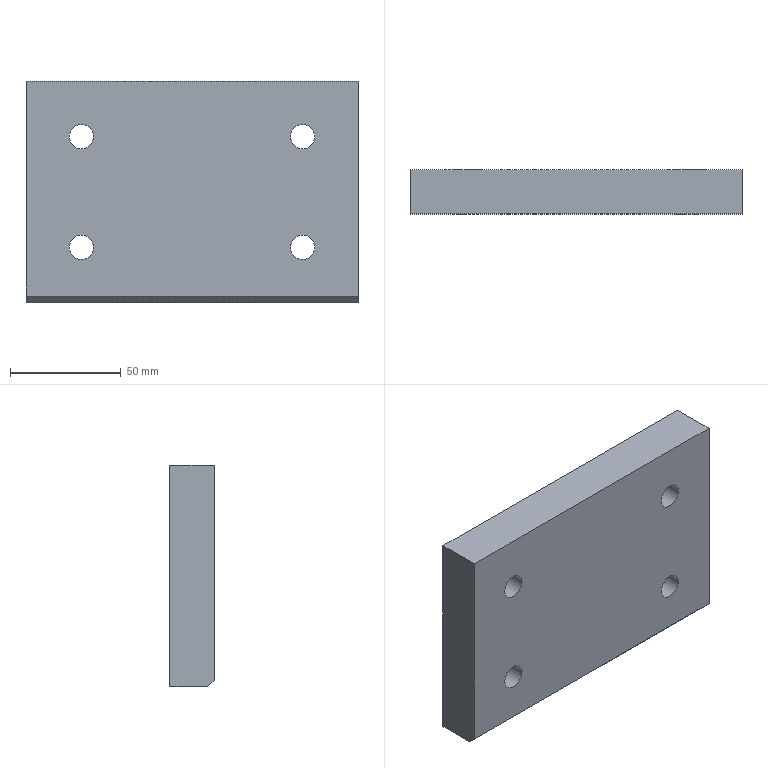Part | NX | features 103 2 | 1 solid | 19 faces | box 150 x 20 x 100 mm | volume 284739 mm3 | plane 11 | cylinder 8 | commonest cylinder face diameters 11 x4 17.5 x4
STEP:
#1=CARTESIAN_POINT('',(-1488.75,770.,-50.));
#2=VERTEX_POINT('',#1);
#3=CARTESIAN_POINT('',(-1480.,770.,-50.));
#4=DIRECTION('',(0.,1.,0.));
#5=DIRECTION('',(-1.,0.,0.));
#6=AXIS2_PLACEMENT_3D('',#3,#4,#5);
#7=CIRCLE('',#6,8.75);
#8=EDGE_CURVE('',#2,#2,#7,.T.);
#9=ORIENTED_EDGE('',*,*,#8,.F.);
#10=EDGE_LOOP('',(#9));
#11=FACE_BOUND('',#10,.T.);
#12=CARTESIAN_POINT('',(-1571.25,770.,0.000000001));
#13=VERTEX_POINT('',#12);
#14=CARTESIAN_POINT('',(-1580.,770.,0.000000001));
#15=DIRECTION('',(0.,-1.,0.));
#16=DIRECTION('',(1.,0.,0.));
#17=AXIS2_PLACEMENT_3D('',#14,#15,#16);
#18=CIRCLE('',#17,8.75);
#19=EDGE_CURVE('',#13,#13,#18,.F.);
#20=ORIENTED_EDGE('',*,*,#19,.F.);
#21=EDGE_LOOP('',(#20));
#22=FACE_BOUND('',#21,.T.);
#23=CARTESIAN_POINT('',(-1571.25,770.,-50.));
#24=VERTEX_POINT('',#23);
#25=CARTESIAN_POINT('',(-1580.,770.,-50.));
#26=DIRECTION('',(0.,-1.,0.));
#27=DIRECTION('',(1.,0.,0.));
#28=AXIS2_PLACEMENT_3D('',#25,#26,#27);
#29=CIRCLE('',#28,8.75);
#30=EDGE_CURVE('',#24,#24,#29,.F.);
#31=ORIENTED_EDGE('',*,*,#30,.F.);
#32=EDGE_LOOP('',(#31));
#33=FACE_BOUND('',#32,.T.);
#34=CARTESIAN_POINT('',(-1471.25,770.,0.000000001));
#35=VERTEX_POINT('',#34);
#36=CARTESIAN_POINT('',(-1480.,770.,0.000000001));
#37=DIRECTION('',(0.,-1.,0.));
#38=DIRECTION('',(1.,0.,0.));
#39=AXIS2_PLACEMENT_3D('',#36,#37,#38);
#40=CIRCLE('',#39,8.75);
#41=EDGE_CURVE('',#35,#35,#40,.F.);
#42=ORIENTED_EDGE('',*,*,#41,.F.);
#43=EDGE_LOOP('',(#42));
#44=FACE_BOUND('',#43,.T.);
#45=CARTESIAN_POINT('',(-1455.,770.,25.));
#46=VERTEX_POINT('',#45);
#47=CARTESIAN_POINT('',(-1455.,770.,-75.));
#48=VERTEX_POINT('',#47);
#49=CARTESIAN_POINT('',(-1455.,770.,-25.));
#50=DIRECTION('',(0.,0.,-1.));
#51=VECTOR('',#50,1000.);
#52=LINE('',#49,#51);
#53=EDGE_CURVE('',#46,#48,#52,.T.);
#54=ORIENTED_EDGE('',*,*,#53,.T.);
#55=CARTESIAN_POINT('',(-1605.,770.,-75.));
#56=VERTEX_POINT('',#55);
#57=CARTESIAN_POINT('',(-1530.,770.,-75.));
#58=DIRECTION('',(-1.,0.,0.));
#59=VECTOR('',#58,1000.);
#60=LINE('',#57,#59);
#61=EDGE_CURVE('',#48,#56,#60,.T.);
#62=ORIENTED_EDGE('',*,*,#61,.T.);
#63=CARTESIAN_POINT('',(-1605.,770.,25.));
#64=VERTEX_POINT('',#63);
#65=CARTESIAN_POINT('',(-1605.,770.,-25.));
#66=DIRECTION('',(0.,0.,1.));
#67=VECTOR('',#66,1000.);
#68=LINE('',#65,#67);
#69=EDGE_CURVE('',#56,#64,#68,.T.);
#70=ORIENTED_EDGE('',*,*,#69,.T.);
#71=CARTESIAN_POINT('',(-1530.,770.,25.));
#72=DIRECTION('',(1.,0.,0.));
#73=VECTOR('',#72,1000.);
#74=LINE('',#71,#73);
#75=EDGE_CURVE('',#64,#46,#74,.T.);
#76=ORIENTED_EDGE('',*,*,#75,.T.);
#77=EDGE_LOOP('',(#54,#62,#70,#76));
#78=FACE_BOUND('',#77,.T.);
#79=CARTESIAN_POINT('',(-1530.,770.,-25.));
#80=DIRECTION('',(0.,1.,0.));
#81=DIRECTION('',(1.,0.,0.));
#82=AXIS2_PLACEMENT_3D('',#79,#80,#81);
#83=PLANE('',#82);
#84=ADVANCED_FACE('',(#11,#22,#33,#44,#78),#83,.T.);
#85=CARTESIAN_POINT('',(-1605.,753.,-75.));
#86=VERTEX_POINT('',#85);
#87=CARTESIAN_POINT('',(-1605.,750.,-75.));
#88=DIRECTION('',(0.,1.,0.));
#89=VECTOR('',#88,1000.);
#90=LINE('',#87,#89);
#91=EDGE_CURVE('',#86,#56,#90,.T.);
#92=ORIENTED_EDGE('',*,*,#91,.T.);
#93=ORIENTED_EDGE('',*,*,#61,.F.);
#94=CARTESIAN_POINT('',(-1455.,753.,-75.));
#95=VERTEX_POINT('',#94);
#96=CARTESIAN_POINT('',(-1455.,750.,-75.));
#97=DIRECTION('',(0.,1.,0.));
#98=VECTOR('',#97,1000.);
#99=LINE('',#96,#98);
#100=EDGE_CURVE('',#95,#48,#99,.T.);
#101=ORIENTED_EDGE('',*,*,#100,.F.);
#102=CARTESIAN_POINT('',(-1530.,753.,-75.));
#103=DIRECTION('',(1.,0.,0.));
#104=VECTOR('',#103,1000.);
#105=LINE('',#102,#104);
#106=EDGE_CURVE('',#86,#95,#105,.T.);
#107=ORIENTED_EDGE('',*,*,#106,.F.);
#108=EDGE_LOOP('',(#92,#93,#101,#107));
#109=FACE_BOUND('',#108,.T.);
#110=CARTESIAN_POINT('',(-1530.,750.,-75.));
#111=DIRECTION('',(0.,0.,-1.));
#112=DIRECTION('',(0.,-1.,0.));
#113=AXIS2_PLACEMENT_3D('',#110,#111,#112);
#114=PLANE('',#113);
#115=ADVANCED_FACE('',(#109),#114,.T.);
#116=CARTESIAN_POINT('',(-1605.,750.,25.));
#117=VERTEX_POINT('',#116);
#118=CARTESIAN_POINT('',(-1605.,750.,-72.));
#119=VERTEX_POINT('',#118);
#120=CARTESIAN_POINT('',(-1605.,750.,-25.));
#121=DIRECTION('',(0.,0.,-1.));
#122=VECTOR('',#121,1000.);
#123=LINE('',#120,#122);
#124=EDGE_CURVE('',#117,#119,#123,.T.);
#125=ORIENTED_EDGE('',*,*,#124,.F.);
#126=CARTESIAN_POINT('',(-1605.,750.,25.));
#127=DIRECTION('',(0.,1.,0.));
#128=VECTOR('',#127,1000.);
#129=LINE('',#126,#128);
#130=EDGE_CURVE('',#117,#64,#129,.T.);
#131=ORIENTED_EDGE('',*,*,#130,.T.);
#132=ORIENTED_EDGE('',*,*,#69,.F.);
#133=ORIENTED_EDGE('',*,*,#91,.F.);
#134=CARTESIAN_POINT('',(-1605.,726.5,-48.5));
#135=DIRECTION('',(0.,-0.7071,0.7071));
#136=VECTOR('',#135,1000.);
#137=LINE('',#134,#136);
#138=EDGE_CURVE('',#119,#86,#137,.F.);
#139=ORIENTED_EDGE('',*,*,#138,.F.);
#140=EDGE_LOOP('',(#125,#131,#132,#133,#139));
#141=FACE_BOUND('',#140,.T.);
#142=CARTESIAN_POINT('',(-1605.,750.,-25.));
#143=DIRECTION('',(-1.,0.,0.));
#144=DIRECTION('',(0.,1.,0.));
#145=AXIS2_PLACEMENT_3D('',#142,#143,#144);
#146=PLANE('',#145);
#147=ADVANCED_FACE('',(#141),#146,.T.);
#148=ORIENTED_EDGE('',*,*,#130,.F.);
#149=CARTESIAN_POINT('',(-1455.,750.,25.));
#150=VERTEX_POINT('',#149);
#151=CARTESIAN_POINT('',(-1530.,750.,25.));
#152=DIRECTION('',(-1.,0.,0.));
#153=VECTOR('',#152,1000.);
#154=LINE('',#151,#153);
#155=EDGE_CURVE('',#150,#117,#154,.T.);
#156=ORIENTED_EDGE('',*,*,#155,.F.);
#157=CARTESIAN_POINT('',(-1455.,750.,25.));
#158=DIRECTION('',(0.,1.,0.));
#159=VECTOR('',#158,1000.);
#160=LINE('',#157,#159);
#161=EDGE_CURVE('',#150,#46,#160,.T.);
#162=ORIENTED_EDGE('',*,*,#161,.T.);
#163=ORIENTED_EDGE('',*,*,#75,.F.);
#164=EDGE_LOOP('',(#148,#156,#162,#163));
#165=FACE_BOUND('',#164,.T.);
#166=CARTESIAN_POINT('',(-1530.,750.,25.));
#167=DIRECTION('',(0.,0.,1.));
#168=DIRECTION('',(0.,1.,0.));
#169=AXIS2_PLACEMENT_3D('',#166,#167,#168);
#170=PLANE('',#169);
#171=ADVANCED_FACE('',(#165),#170,.T.);
#172=CARTESIAN_POINT('',(-1485.5,750.,-50.));
#173=VERTEX_POINT('',#172);
#174=CARTESIAN_POINT('',(-1480.,750.,-50.));
#175=DIRECTION('',(0.,1.,0.));
#176=DIRECTION('',(-1.,0.,0.));
#177=AXIS2_PLACEMENT_3D('',#174,#175,#176);
#178=CIRCLE('',#177,5.5);
#179=EDGE_CURVE('',#173,#173,#178,.T.);
#180=ORIENTED_EDGE('',*,*,#179,.T.);
#181=EDGE_LOOP('',(#180));
#182=FACE_BOUND('',#181,.T.);
#183=CARTESIAN_POINT('',(-1585.5,750.,0.000000001));
#184=VERTEX_POINT('',#183);
#185=CARTESIAN_POINT('',(-1580.,750.,0.000000001));
#186=DIRECTION('',(0.,1.,0.));
#187=DIRECTION('',(-1.,0.,0.));
#188=AXIS2_PLACEMENT_3D('',#185,#186,#187);
#189=CIRCLE('',#188,5.5);
#190=EDGE_CURVE('',#184,#184,#189,.T.);
#191=ORIENTED_EDGE('',*,*,#190,.T.);
#192=EDGE_LOOP('',(#191));
#193=FACE_BOUND('',#192,.T.);
#194=CARTESIAN_POINT('',(-1585.5,750.,-50.));
#195=VERTEX_POINT('',#194);
#196=CARTESIAN_POINT('',(-1580.,750.,-50.));
#197=DIRECTION('',(0.,1.,0.));
#198=DIRECTION('',(-1.,0.,0.));
#199=AXIS2_PLACEMENT_3D('',#196,#197,#198);
#200=CIRCLE('',#199,5.5);
#201=EDGE_CURVE('',#195,#195,#200,.F.);
#202=ORIENTED_EDGE('',*,*,#201,.F.);
#203=EDGE_LOOP('',(#202));
#204=FACE_BOUND('',#203,.T.);
#205=CARTESIAN_POINT('',(-1485.5,750.,0.000000001));
#206=VERTEX_POINT('',#205);
#207=CARTESIAN_POINT('',(-1480.,750.,0.000000001));
#208=DIRECTION('',(0.,1.,0.));
#209=DIRECTION('',(-1.,0.,0.));
#210=AXIS2_PLACEMENT_3D('',#207,#208,#209);
#211=CIRCLE('',#210,5.5);
#212=EDGE_CURVE('',#206,#206,#211,.F.);
#213=ORIENTED_EDGE('',*,*,#212,.F.);
#214=EDGE_LOOP('',(#213));
#215=FACE_BOUND('',#214,.T.);
#216=CARTESIAN_POINT('',(-1455.,750.,-72.));
#217=VERTEX_POINT('',#216);
#218=CARTESIAN_POINT('',(-1455.,750.,-25.));
#219=DIRECTION('',(0.,0.,1.));
#220=VECTOR('',#219,1000.);
#221=LINE('',#218,#220);
#222=EDGE_CURVE('',#217,#150,#221,.T.);
#223=ORIENTED_EDGE('',*,*,#222,.T.);
#224=ORIENTED_EDGE('',*,*,#155,.T.);
#225=ORIENTED_EDGE('',*,*,#124,.T.);
#226=CARTESIAN_POINT('',(-1530.,750.,-72.));
#227=DIRECTION('',(-1.,0.,0.));
#228=VECTOR('',#227,1000.);
#229=LINE('',#226,#228);
#230=EDGE_CURVE('',#217,#119,#229,.T.);
#231=ORIENTED_EDGE('',*,*,#230,.F.);
#232=EDGE_LOOP('',(#223,#224,#225,#231));
#233=FACE_BOUND('',#232,.T.);
#234=CARTESIAN_POINT('',(-1530.,750.,-25.));
#235=DIRECTION('',(0.,-1.,0.));
#236=DIRECTION('',(-1.,0.,0.));
#237=AXIS2_PLACEMENT_3D('',#234,#235,#236);
#238=PLANE('',#237);
#239=ADVANCED_FACE('',(#182,#193,#204,#215,#233),#238,.T.);
#240=ORIENTED_EDGE('',*,*,#100,.T.);
#241=ORIENTED_EDGE('',*,*,#53,.F.);
#242=ORIENTED_EDGE('',*,*,#161,.F.);
#243=ORIENTED_EDGE('',*,*,#222,.F.);
#244=CARTESIAN_POINT('',(-1455.,726.5,-48.5));
#245=DIRECTION('',(0.,0.7071,-0.7071));
#246=VECTOR('',#245,1000.);
#247=LINE('',#244,#246);
#248=EDGE_CURVE('',#95,#217,#247,.F.);
#249=ORIENTED_EDGE('',*,*,#248,.F.);
#250=EDGE_LOOP('',(#240,#241,#242,#243,#249));
#251=FACE_BOUND('',#250,.T.);
#252=CARTESIAN_POINT('',(-1455.,750.,-25.));
#253=DIRECTION('',(1.,0.,0.));
#254=DIRECTION('',(0.,-1.,0.));
#255=AXIS2_PLACEMENT_3D('',#252,#253,#254);
#256=PLANE('',#255);
#257=ADVANCED_FACE('',(#251),#256,.T.);
#258=ORIENTED_EDGE('',*,*,#138,.T.);
#259=ORIENTED_EDGE('',*,*,#106,.T.);
#260=ORIENTED_EDGE('',*,*,#248,.T.);
#261=ORIENTED_EDGE('',*,*,#230,.T.);
#262=EDGE_LOOP('',(#258,#259,#260,#261));
#263=FACE_BOUND('',#262,.T.);
#264=CARTESIAN_POINT('',(-1530.,753.,-75.));
#265=DIRECTION('',(0.,0.7071,0.7071));
#266=DIRECTION('',(0.,0.7071,-0.7071));
#267=AXIS2_PLACEMENT_3D('',#264,#265,#266);
#268=PLANE('',#267);
#269=ADVANCED_FACE('',(#263),#268,.F.);
#270=CARTESIAN_POINT('',(-1485.5,758.,0.000000001));
#271=VERTEX_POINT('',#270);
#272=CARTESIAN_POINT('',(-1480.,758.,0.000000001));
#273=DIRECTION('',(0.,1.,0.));
#274=DIRECTION('',(-1.,0.,0.));
#275=AXIS2_PLACEMENT_3D('',#272,#273,#274);
#276=CIRCLE('',#275,5.5);
#277=EDGE_CURVE('',#271,#271,#276,.F.);
#278=ORIENTED_EDGE('',*,*,#277,.F.);
#279=EDGE_LOOP('',(#278));
#280=FACE_BOUND('',#279,.T.);
#281=ORIENTED_EDGE('',*,*,#212,.T.);
#282=EDGE_LOOP('',(#281));
#283=FACE_BOUND('',#282,.T.);
#284=CARTESIAN_POINT('',(-1480.,750.,0.000000001));
#285=DIRECTION('',(0.,1.,0.));
#286=DIRECTION('',(0.,0.,-1.));
#287=AXIS2_PLACEMENT_3D('',#284,#285,#286);
#288=CYLINDRICAL_SURFACE('',#287,5.5);
#289=ADVANCED_FACE('',(#280,#283),#288,.F.);
#290=CARTESIAN_POINT('',(-1585.5,758.,-50.));
#291=VERTEX_POINT('',#290);
#292=CARTESIAN_POINT('',(-1580.,758.,-50.));
#293=DIRECTION('',(0.,1.,0.));
#294=DIRECTION('',(-1.,0.,0.));
#295=AXIS2_PLACEMENT_3D('',#292,#293,#294);
#296=CIRCLE('',#295,5.5);
#297=EDGE_CURVE('',#291,#291,#296,.F.);
#298=ORIENTED_EDGE('',*,*,#297,.F.);
#299=EDGE_LOOP('',(#298));
#300=FACE_BOUND('',#299,.T.);
#301=ORIENTED_EDGE('',*,*,#201,.T.);
#302=EDGE_LOOP('',(#301));
#303=FACE_BOUND('',#302,.T.);
#304=CARTESIAN_POINT('',(-1580.,750.,-50.));
#305=DIRECTION('',(0.,1.,0.));
#306=DIRECTION('',(0.,0.,-1.));
#307=AXIS2_PLACEMENT_3D('',#304,#305,#306);
#308=CYLINDRICAL_SURFACE('',#307,5.5);
#309=ADVANCED_FACE('',(#300,#303),#308,.F.);
#310=CARTESIAN_POINT('',(-1488.75,758.,0.000000001));
#311=VERTEX_POINT('',#310);
#312=CARTESIAN_POINT('',(-1480.,758.,0.000000001));
#313=DIRECTION('',(0.,1.,0.));
#314=DIRECTION('',(-1.,0.,0.));
#315=AXIS2_PLACEMENT_3D('',#312,#313,#314);
#316=CIRCLE('',#315,8.75);
#317=EDGE_CURVE('',#311,#311,#316,.F.);
#318=ORIENTED_EDGE('',*,*,#317,.F.);
#319=EDGE_LOOP('',(#318));
#320=FACE_BOUND('',#319,.T.);
#321=ORIENTED_EDGE('',*,*,#277,.T.);
#322=EDGE_LOOP('',(#321));
#323=FACE_BOUND('',#322,.T.);
#324=CARTESIAN_POINT('',(-1475.,758.,100.));
#325=DIRECTION('',(0.,-1.,0.));
#326=DIRECTION('',(0.,0.,1.));
#327=AXIS2_PLACEMENT_3D('',#324,#325,#326);
#328=PLANE('',#327);
#329=ADVANCED_FACE('',(#320,#323),#328,.F.);
#330=ORIENTED_EDGE('',*,*,#317,.T.);
#331=EDGE_LOOP('',(#330));
#332=FACE_BOUND('',#331,.T.);
#333=ORIENTED_EDGE('',*,*,#41,.T.);
#334=EDGE_LOOP('',(#333));
#335=FACE_BOUND('',#334,.T.);
#336=CARTESIAN_POINT('',(-1480.,770.,0.000000001));
#337=DIRECTION('',(0.,-1.,0.));
#338=DIRECTION('',(0.,0.,1.));
#339=AXIS2_PLACEMENT_3D('',#336,#337,#338);
#340=CYLINDRICAL_SURFACE('',#339,8.75);
#341=ADVANCED_FACE('',(#332,#335),#340,.F.);
#342=CARTESIAN_POINT('',(-1588.75,758.,-50.));
#343=VERTEX_POINT('',#342);
#344=CARTESIAN_POINT('',(-1580.,758.,-50.));
#345=DIRECTION('',(0.,1.,0.));
#346=DIRECTION('',(-1.,0.,0.));
#347=AXIS2_PLACEMENT_3D('',#344,#345,#346);
#348=CIRCLE('',#347,8.75);
#349=EDGE_CURVE('',#343,#343,#348,.F.);
#350=ORIENTED_EDGE('',*,*,#349,.F.);
#351=EDGE_LOOP('',(#350));
#352=FACE_BOUND('',#351,.T.);
#353=ORIENTED_EDGE('',*,*,#297,.T.);
#354=EDGE_LOOP('',(#353));
#355=FACE_BOUND('',#354,.T.);
#356=CARTESIAN_POINT('',(-1525.,758.,-50.));
#357=DIRECTION('',(0.,-1.,0.));
#358=DIRECTION('',(0.,0.,1.));
#359=AXIS2_PLACEMENT_3D('',#356,#357,#358);
#360=PLANE('',#359);
#361=ADVANCED_FACE('',(#352,#355),#360,.F.);
#362=ORIENTED_EDGE('',*,*,#349,.T.);
#363=EDGE_LOOP('',(#362));
#364=FACE_BOUND('',#363,.T.);
#365=ORIENTED_EDGE('',*,*,#30,.T.);
#366=EDGE_LOOP('',(#365));
#367=FACE_BOUND('',#366,.T.);
#368=CARTESIAN_POINT('',(-1580.,770.,-50.));
#369=DIRECTION('',(0.,-1.,0.));
#370=DIRECTION('',(0.,0.,1.));
#371=AXIS2_PLACEMENT_3D('',#368,#369,#370);
#372=CYLINDRICAL_SURFACE('',#371,8.75);
#373=ADVANCED_FACE('',(#364,#367),#372,.F.);
#374=CARTESIAN_POINT('',(-1585.5,758.,0.000000001));
#375=VERTEX_POINT('',#374);
#376=CARTESIAN_POINT('',(-1580.,758.,0.000000001));
#377=DIRECTION('',(0.,1.,0.));
#378=DIRECTION('',(-1.,0.,0.));
#379=AXIS2_PLACEMENT_3D('',#376,#377,#378);
#380=CIRCLE('',#379,5.5);
#381=EDGE_CURVE('',#375,#375,#380,.T.);
#382=ORIENTED_EDGE('',*,*,#381,.F.);
#383=EDGE_LOOP('',(#382));
#384=FACE_BOUND('',#383,.T.);
#385=CARTESIAN_POINT('',(-1588.75,758.,0.000000001));
#386=VERTEX_POINT('',#385);
#387=CARTESIAN_POINT('',(-1580.,758.,0.000000001));
#388=DIRECTION('',(0.,1.,0.));
#389=DIRECTION('',(-1.,0.,0.));
#390=AXIS2_PLACEMENT_3D('',#387,#388,#389);
#391=CIRCLE('',#390,8.75);
#392=EDGE_CURVE('',#386,#386,#391,.F.);
#393=ORIENTED_EDGE('',*,*,#392,.F.);
#394=EDGE_LOOP('',(#393));
#395=FACE_BOUND('',#394,.T.);
#396=CARTESIAN_POINT('',(-1585.,758.,100.));
#397=DIRECTION('',(0.,-1.,0.));
#398=DIRECTION('',(0.,0.,1.));
#399=AXIS2_PLACEMENT_3D('',#396,#397,#398);
#400=PLANE('',#399);
#401=ADVANCED_FACE('',(#384,#395),#400,.F.);
#402=ORIENTED_EDGE('',*,*,#392,.T.);
#403=EDGE_LOOP('',(#402));
#404=FACE_BOUND('',#403,.T.);
#405=ORIENTED_EDGE('',*,*,#19,.T.);
#406=EDGE_LOOP('',(#405));
#407=FACE_BOUND('',#406,.T.);
#408=CARTESIAN_POINT('',(-1580.,770.,0.000000001));
#409=DIRECTION('',(0.,-1.,0.));
#410=DIRECTION('',(0.,0.,1.));
#411=AXIS2_PLACEMENT_3D('',#408,#409,#410);
#412=CYLINDRICAL_SURFACE('',#411,8.75);
#413=ADVANCED_FACE('',(#404,#407),#412,.F.);
#414=ORIENTED_EDGE('',*,*,#190,.F.);
#415=EDGE_LOOP('',(#414));
#416=FACE_BOUND('',#415,.T.);
#417=ORIENTED_EDGE('',*,*,#381,.T.);
#418=EDGE_LOOP('',(#417));
#419=FACE_BOUND('',#418,.T.);
#420=CARTESIAN_POINT('',(-1580.,757.,0.000000001));
#421=DIRECTION('',(0.,-1.,0.));
#422=DIRECTION('',(0.,0.,1.));
#423=AXIS2_PLACEMENT_3D('',#420,#421,#422);
#424=CYLINDRICAL_SURFACE('',#423,5.5);
#425=ADVANCED_FACE('',(#416,#419),#424,.F.);
#426=ORIENTED_EDGE('',*,*,#179,.F.);
#427=EDGE_LOOP('',(#426));
#428=FACE_BOUND('',#427,.T.);
#429=CARTESIAN_POINT('',(-1485.5,758.,-50.));
#430=VERTEX_POINT('',#429);
#431=CARTESIAN_POINT('',(-1480.,758.,-50.));
#432=DIRECTION('',(0.,1.,0.));
#433=DIRECTION('',(-1.,0.,0.));
#434=AXIS2_PLACEMENT_3D('',#431,#432,#433);
#435=CIRCLE('',#434,5.5);
#436=EDGE_CURVE('',#430,#430,#435,.T.);
#437=ORIENTED_EDGE('',*,*,#436,.T.);
#438=EDGE_LOOP('',(#437));
#439=FACE_BOUND('',#438,.T.);
#440=CARTESIAN_POINT('',(-1480.,720.,-50.));
#441=DIRECTION('',(0.,-1.,0.));
#442=DIRECTION('',(-1.,0.,0.));
#443=AXIS2_PLACEMENT_3D('',#440,#441,#442);
#444=CYLINDRICAL_SURFACE('',#443,5.5);
#445=ADVANCED_FACE('',(#428,#439),#444,.F.);
#446=ORIENTED_EDGE('',*,*,#436,.F.);
#447=EDGE_LOOP('',(#446));
#448=FACE_BOUND('',#447,.T.);
#449=CARTESIAN_POINT('',(-1488.75,758.,-50.));
#450=VERTEX_POINT('',#449);
#451=CARTESIAN_POINT('',(-1480.,758.,-50.));
#452=DIRECTION('',(0.,1.,0.));
#453=DIRECTION('',(-1.,0.,0.));
#454=AXIS2_PLACEMENT_3D('',#451,#452,#453);
#455=CIRCLE('',#454,8.75);
#456=EDGE_CURVE('',#450,#450,#455,.T.);
#457=ORIENTED_EDGE('',*,*,#456,.T.);
#458=EDGE_LOOP('',(#457));
#459=FACE_BOUND('',#458,.T.);
#460=CARTESIAN_POINT('',(-1475.,758.,-50.));
#461=DIRECTION('',(0.,-1.,0.));
#462=DIRECTION('',(-1.,0.,0.));
#463=AXIS2_PLACEMENT_3D('',#460,#461,#462);
#464=PLANE('',#463);
#465=ADVANCED_FACE('',(#448,#459),#464,.F.);
#466=ORIENTED_EDGE('',*,*,#456,.F.);
#467=EDGE_LOOP('',(#466));
#468=FACE_BOUND('',#467,.T.);
#469=ORIENTED_EDGE('',*,*,#8,.T.);
#470=EDGE_LOOP('',(#469));
#471=FACE_BOUND('',#470,.T.);
#472=CARTESIAN_POINT('',(-1480.,770.,-50.));
#473=DIRECTION('',(0.,-1.,0.));
#474=DIRECTION('',(-1.,0.,0.));
#475=AXIS2_PLACEMENT_3D('',#472,#473,#474);
#476=CYLINDRICAL_SURFACE('',#475,8.75);
#477=ADVANCED_FACE('',(#468,#471),#476,.F.);
#478=CLOSED_SHELL('',(#84,#115,#147,#171,#239,#257,#269,#289,#309,#329,#341,#361,#373,#401,#413,#425,#445,#465,#477));
#479=MANIFOLD_SOLID_BREP('',#478);
#480=(LENGTH_UNIT()NAMED_UNIT(*)SI_UNIT(.MILLI.,.METRE.));
#481=UNCERTAINTY_MEASURE_WITH_UNIT(LENGTH_MEASURE(0.00001),#480,'','');
#482=(NAMED_UNIT(*)PLANE_ANGLE_UNIT()SI_UNIT($,.RADIAN.));
#483=(NAMED_UNIT(*)SI_UNIT($,.STERADIAN.)SOLID_ANGLE_UNIT());
#484=(GEOMETRIC_REPRESENTATION_CONTEXT(3)GLOBAL_UNCERTAINTY_ASSIGNED_CONTEXT((#481))GLOBAL_UNIT_ASSIGNED_CONTEXT((#480,#482,#483))REPRESENTATION_CONTEXT('',''));
#485=ADVANCED_BREP_SHAPE_REPRESENTATION('',(#479),#484);